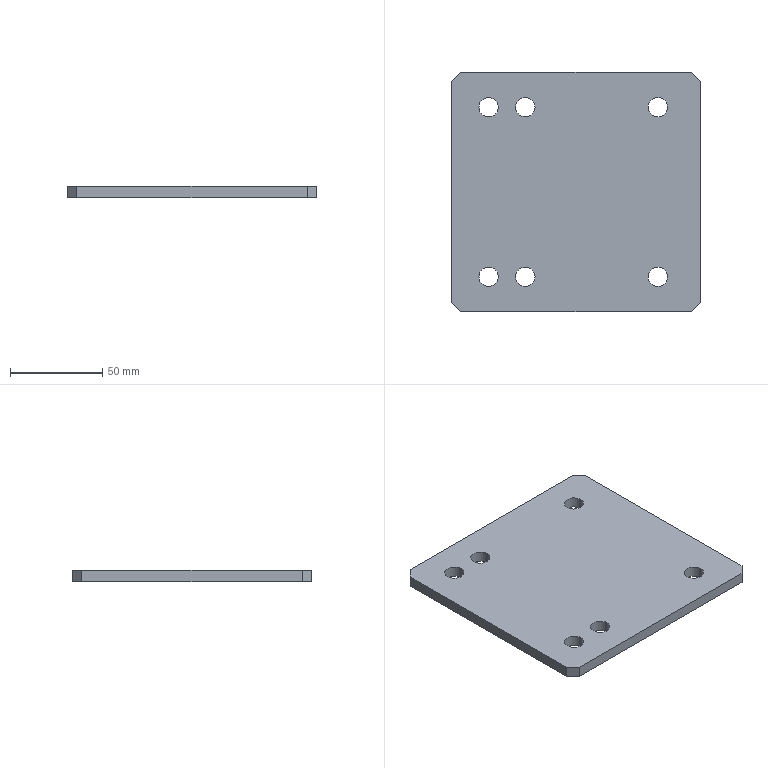Part | SolidWorks | features Extrusion 1 | 1 solid | 22 faces | box 135 x 130 x 6 mm | volume 101883 mm3 | cylinder 12 | plane 10 | commonest cylinder face diameters 10.5 x12
STEP:
#1=CARTESIAN_POINT('',(-52.75,-46.,3.));
#2=VERTEX_POINT('',#1);
#3=CARTESIAN_POINT('',(-42.25,-46.,3.));
#4=VERTEX_POINT('',#3);
#5=CARTESIAN_POINT('',(-47.5,-46.,3.));
#6=DIRECTION('',(0.,0.,1.));
#7=DIRECTION('',(-1.,0.,0.));
#8=AXIS2_PLACEMENT_3D('',#5,#6,#7);
#9=CIRCLE('',#8,5.25);
#10=EDGE_CURVE('',#2,#4,#9,.T.);
#11=ORIENTED_EDGE('',*,*,#10,.T.);
#12=CARTESIAN_POINT('',(-42.25,-46.,-3.));
#13=VERTEX_POINT('',#12);
#14=CARTESIAN_POINT('',(-42.25,-46.,3.));
#15=DIRECTION('',(0.,0.,-1.));
#16=VECTOR('',#15,1000.);
#17=LINE('',#14,#16);
#18=EDGE_CURVE('',#4,#13,#17,.T.);
#19=ORIENTED_EDGE('',*,*,#18,.T.);
#20=CARTESIAN_POINT('',(-52.75,-46.,-3.));
#21=VERTEX_POINT('',#20);
#22=CARTESIAN_POINT('',(-47.5,-46.,-3.));
#23=DIRECTION('',(0.,0.,1.));
#24=DIRECTION('',(-1.,0.,0.));
#25=AXIS2_PLACEMENT_3D('',#22,#23,#24);
#26=CIRCLE('',#25,5.25);
#27=EDGE_CURVE('',#21,#13,#26,.T.);
#28=ORIENTED_EDGE('',*,*,#27,.F.);
#29=CARTESIAN_POINT('',(-52.75,-46.,3.));
#30=DIRECTION('',(0.,0.,-1.));
#31=VECTOR('',#30,1000.);
#32=LINE('',#29,#31);
#33=EDGE_CURVE('',#2,#21,#32,.T.);
#34=ORIENTED_EDGE('',*,*,#33,.F.);
#35=EDGE_LOOP('',(#11,#19,#28,#34));
#36=FACE_OUTER_BOUND('',#35,.T.);
#37=CARTESIAN_POINT('',(-47.5,-46.,3.));
#38=DIRECTION('',(0.,0.,-1.));
#39=DIRECTION('',(-1.,0.,0.));
#40=AXIS2_PLACEMENT_3D('',#37,#38,#39);
#41=CYLINDRICAL_SURFACE('',#40,5.25);
#42=ADVANCED_FACE('',(#36),#41,.F.);
#43=CARTESIAN_POINT('',(-32.75,-46.,3.));
#44=VERTEX_POINT('',#43);
#45=CARTESIAN_POINT('',(-22.25,-46.,3.));
#46=VERTEX_POINT('',#45);
#47=CARTESIAN_POINT('',(-27.5,-46.,3.));
#48=DIRECTION('',(0.,0.,1.));
#49=DIRECTION('',(-1.,0.,0.));
#50=AXIS2_PLACEMENT_3D('',#47,#48,#49);
#51=CIRCLE('',#50,5.25);
#52=EDGE_CURVE('',#44,#46,#51,.T.);
#53=ORIENTED_EDGE('',*,*,#52,.T.);
#54=CARTESIAN_POINT('',(-22.25,-46.,-3.));
#55=VERTEX_POINT('',#54);
#56=CARTESIAN_POINT('',(-22.25,-46.,3.));
#57=DIRECTION('',(0.,0.,-1.));
#58=VECTOR('',#57,1000.);
#59=LINE('',#56,#58);
#60=EDGE_CURVE('',#46,#55,#59,.T.);
#61=ORIENTED_EDGE('',*,*,#60,.T.);
#62=CARTESIAN_POINT('',(-32.75,-46.,-3.));
#63=VERTEX_POINT('',#62);
#64=CARTESIAN_POINT('',(-27.5,-46.,-3.));
#65=DIRECTION('',(0.,0.,1.));
#66=DIRECTION('',(-1.,0.,0.));
#67=AXIS2_PLACEMENT_3D('',#64,#65,#66);
#68=CIRCLE('',#67,5.25);
#69=EDGE_CURVE('',#63,#55,#68,.T.);
#70=ORIENTED_EDGE('',*,*,#69,.F.);
#71=CARTESIAN_POINT('',(-32.75,-46.,3.));
#72=DIRECTION('',(0.,0.,-1.));
#73=VECTOR('',#72,1000.);
#74=LINE('',#71,#73);
#75=EDGE_CURVE('',#44,#63,#74,.T.);
#76=ORIENTED_EDGE('',*,*,#75,.F.);
#77=EDGE_LOOP('',(#53,#61,#70,#76));
#78=FACE_OUTER_BOUND('',#77,.T.);
#79=CARTESIAN_POINT('',(-27.5,-46.,3.));
#80=DIRECTION('',(0.,0.,-1.));
#81=DIRECTION('',(-1.,0.,0.));
#82=AXIS2_PLACEMENT_3D('',#79,#80,#81);
#83=CYLINDRICAL_SURFACE('',#82,5.25);
#84=ADVANCED_FACE('',(#78),#83,.F.);
#85=CARTESIAN_POINT('',(39.25,-46.,3.));
#86=VERTEX_POINT('',#85);
#87=CARTESIAN_POINT('',(49.75,-46.,3.));
#88=VERTEX_POINT('',#87);
#89=CARTESIAN_POINT('',(44.5,-46.,3.));
#90=DIRECTION('',(0.,0.,1.));
#91=DIRECTION('',(-1.,0.,0.));
#92=AXIS2_PLACEMENT_3D('',#89,#90,#91);
#93=CIRCLE('',#92,5.25);
#94=EDGE_CURVE('',#86,#88,#93,.T.);
#95=ORIENTED_EDGE('',*,*,#94,.T.);
#96=CARTESIAN_POINT('',(49.75,-46.,-3.));
#97=VERTEX_POINT('',#96);
#98=CARTESIAN_POINT('',(49.75,-46.,3.));
#99=DIRECTION('',(0.,0.,-1.));
#100=VECTOR('',#99,1000.);
#101=LINE('',#98,#100);
#102=EDGE_CURVE('',#88,#97,#101,.T.);
#103=ORIENTED_EDGE('',*,*,#102,.T.);
#104=CARTESIAN_POINT('',(39.25,-46.,-3.));
#105=VERTEX_POINT('',#104);
#106=CARTESIAN_POINT('',(44.5,-46.,-3.));
#107=DIRECTION('',(0.,0.,1.));
#108=DIRECTION('',(-1.,0.,0.));
#109=AXIS2_PLACEMENT_3D('',#106,#107,#108);
#110=CIRCLE('',#109,5.25);
#111=EDGE_CURVE('',#105,#97,#110,.T.);
#112=ORIENTED_EDGE('',*,*,#111,.F.);
#113=CARTESIAN_POINT('',(39.25,-46.,3.));
#114=DIRECTION('',(0.,0.,-1.));
#115=VECTOR('',#114,1000.);
#116=LINE('',#113,#115);
#117=EDGE_CURVE('',#86,#105,#116,.T.);
#118=ORIENTED_EDGE('',*,*,#117,.F.);
#119=EDGE_LOOP('',(#95,#103,#112,#118));
#120=FACE_OUTER_BOUND('',#119,.T.);
#121=CARTESIAN_POINT('',(44.5,-46.,3.));
#122=DIRECTION('',(0.,0.,-1.));
#123=DIRECTION('',(-1.,0.,0.));
#124=AXIS2_PLACEMENT_3D('',#121,#122,#123);
#125=CYLINDRICAL_SURFACE('',#124,5.25);
#126=ADVANCED_FACE('',(#120),#125,.F.);
#127=CARTESIAN_POINT('',(39.25,46.,3.));
#128=VERTEX_POINT('',#127);
#129=CARTESIAN_POINT('',(49.75,46.,3.));
#130=VERTEX_POINT('',#129);
#131=CARTESIAN_POINT('',(44.5,46.,3.));
#132=DIRECTION('',(0.,0.,1.));
#133=DIRECTION('',(1.,0.,0.));
#134=AXIS2_PLACEMENT_3D('',#131,#132,#133);
#135=CIRCLE('',#134,5.25);
#136=EDGE_CURVE('',#128,#130,#135,.T.);
#137=ORIENTED_EDGE('',*,*,#136,.T.);
#138=CARTESIAN_POINT('',(49.75,46.,-3.));
#139=VERTEX_POINT('',#138);
#140=CARTESIAN_POINT('',(49.75,46.,3.));
#141=DIRECTION('',(0.,0.,-1.));
#142=VECTOR('',#141,1000.);
#143=LINE('',#140,#142);
#144=EDGE_CURVE('',#130,#139,#143,.T.);
#145=ORIENTED_EDGE('',*,*,#144,.T.);
#146=CARTESIAN_POINT('',(39.25,46.,-3.));
#147=VERTEX_POINT('',#146);
#148=CARTESIAN_POINT('',(44.5,46.,-3.));
#149=DIRECTION('',(0.,0.,1.));
#150=DIRECTION('',(1.,0.,0.));
#151=AXIS2_PLACEMENT_3D('',#148,#149,#150);
#152=CIRCLE('',#151,5.25);
#153=EDGE_CURVE('',#147,#139,#152,.T.);
#154=ORIENTED_EDGE('',*,*,#153,.F.);
#155=CARTESIAN_POINT('',(39.25,46.,3.));
#156=DIRECTION('',(0.,0.,-1.));
#157=VECTOR('',#156,1000.);
#158=LINE('',#155,#157);
#159=EDGE_CURVE('',#128,#147,#158,.T.);
#160=ORIENTED_EDGE('',*,*,#159,.F.);
#161=EDGE_LOOP('',(#137,#145,#154,#160));
#162=FACE_OUTER_BOUND('',#161,.T.);
#163=CARTESIAN_POINT('',(44.5,46.,3.));
#164=DIRECTION('',(0.,0.,-1.));
#165=DIRECTION('',(-1.,0.,0.));
#166=AXIS2_PLACEMENT_3D('',#163,#164,#165);
#167=CYLINDRICAL_SURFACE('',#166,5.25);
#168=ADVANCED_FACE('',(#162),#167,.F.);
#169=CARTESIAN_POINT('',(-32.75,46.,3.));
#170=VERTEX_POINT('',#169);
#171=CARTESIAN_POINT('',(-22.25,46.,3.));
#172=VERTEX_POINT('',#171);
#173=CARTESIAN_POINT('',(-27.5,46.,3.));
#174=DIRECTION('',(0.,0.,1.));
#175=DIRECTION('',(1.,0.,0.));
#176=AXIS2_PLACEMENT_3D('',#173,#174,#175);
#177=CIRCLE('',#176,5.25);
#178=EDGE_CURVE('',#170,#172,#177,.T.);
#179=ORIENTED_EDGE('',*,*,#178,.T.);
#180=CARTESIAN_POINT('',(-22.25,46.,-3.));
#181=VERTEX_POINT('',#180);
#182=CARTESIAN_POINT('',(-22.25,46.,3.));
#183=DIRECTION('',(0.,0.,-1.));
#184=VECTOR('',#183,1000.);
#185=LINE('',#182,#184);
#186=EDGE_CURVE('',#172,#181,#185,.T.);
#187=ORIENTED_EDGE('',*,*,#186,.T.);
#188=CARTESIAN_POINT('',(-32.75,46.,-3.));
#189=VERTEX_POINT('',#188);
#190=CARTESIAN_POINT('',(-27.5,46.,-3.));
#191=DIRECTION('',(0.,0.,1.));
#192=DIRECTION('',(1.,0.,0.));
#193=AXIS2_PLACEMENT_3D('',#190,#191,#192);
#194=CIRCLE('',#193,5.25);
#195=EDGE_CURVE('',#189,#181,#194,.T.);
#196=ORIENTED_EDGE('',*,*,#195,.F.);
#197=CARTESIAN_POINT('',(-32.75,46.,3.));
#198=DIRECTION('',(0.,0.,-1.));
#199=VECTOR('',#198,1000.);
#200=LINE('',#197,#199);
#201=EDGE_CURVE('',#170,#189,#200,.T.);
#202=ORIENTED_EDGE('',*,*,#201,.F.);
#203=EDGE_LOOP('',(#179,#187,#196,#202));
#204=FACE_OUTER_BOUND('',#203,.T.);
#205=CARTESIAN_POINT('',(-27.5,46.,3.));
#206=DIRECTION('',(0.,0.,-1.));
#207=DIRECTION('',(-1.,0.,0.));
#208=AXIS2_PLACEMENT_3D('',#205,#206,#207);
#209=CYLINDRICAL_SURFACE('',#208,5.25);
#210=ADVANCED_FACE('',(#204),#209,.F.);
#211=CARTESIAN_POINT('',(-52.75,46.,3.));
#212=VERTEX_POINT('',#211);
#213=CARTESIAN_POINT('',(-42.25,46.,3.));
#214=VERTEX_POINT('',#213);
#215=CARTESIAN_POINT('',(-47.5,46.,3.));
#216=DIRECTION('',(0.,0.,1.));
#217=DIRECTION('',(1.,0.,0.));
#218=AXIS2_PLACEMENT_3D('',#215,#216,#217);
#219=CIRCLE('',#218,5.25);
#220=EDGE_CURVE('',#212,#214,#219,.T.);
#221=ORIENTED_EDGE('',*,*,#220,.T.);
#222=CARTESIAN_POINT('',(-42.25,46.,-3.));
#223=VERTEX_POINT('',#222);
#224=CARTESIAN_POINT('',(-42.25,46.,3.));
#225=DIRECTION('',(0.,0.,-1.));
#226=VECTOR('',#225,1000.);
#227=LINE('',#224,#226);
#228=EDGE_CURVE('',#214,#223,#227,.T.);
#229=ORIENTED_EDGE('',*,*,#228,.T.);
#230=CARTESIAN_POINT('',(-52.75,46.,-3.));
#231=VERTEX_POINT('',#230);
#232=CARTESIAN_POINT('',(-47.5,46.,-3.));
#233=DIRECTION('',(0.,0.,1.));
#234=DIRECTION('',(1.,0.,0.));
#235=AXIS2_PLACEMENT_3D('',#232,#233,#234);
#236=CIRCLE('',#235,5.25);
#237=EDGE_CURVE('',#231,#223,#236,.T.);
#238=ORIENTED_EDGE('',*,*,#237,.F.);
#239=CARTESIAN_POINT('',(-52.75,46.,3.));
#240=DIRECTION('',(0.,0.,-1.));
#241=VECTOR('',#240,1000.);
#242=LINE('',#239,#241);
#243=EDGE_CURVE('',#212,#231,#242,.T.);
#244=ORIENTED_EDGE('',*,*,#243,.F.);
#245=EDGE_LOOP('',(#221,#229,#238,#244));
#246=FACE_OUTER_BOUND('',#245,.T.);
#247=CARTESIAN_POINT('',(-47.5,46.,3.));
#248=DIRECTION('',(0.,0.,-1.));
#249=DIRECTION('',(-1.,0.,0.));
#250=AXIS2_PLACEMENT_3D('',#247,#248,#249);
#251=CYLINDRICAL_SURFACE('',#250,5.25);
#252=ADVANCED_FACE('',(#246),#251,.F.);
#253=ORIENTED_EDGE('',*,*,#52,.F.);
#254=CARTESIAN_POINT('',(-27.5,-46.,3.));
#255=DIRECTION('',(0.,0.,1.));
#256=DIRECTION('',(-1.,0.,0.));
#257=AXIS2_PLACEMENT_3D('',#254,#255,#256);
#258=CIRCLE('',#257,5.25);
#259=EDGE_CURVE('',#46,#44,#258,.T.);
#260=ORIENTED_EDGE('',*,*,#259,.F.);
#261=EDGE_LOOP('',(#253,#260));
#262=FACE_BOUND('',#261,.T.);
#263=ORIENTED_EDGE('',*,*,#136,.F.);
#264=CARTESIAN_POINT('',(44.5,46.,3.));
#265=DIRECTION('',(0.,0.,1.));
#266=DIRECTION('',(1.,0.,0.));
#267=AXIS2_PLACEMENT_3D('',#264,#265,#266);
#268=CIRCLE('',#267,5.25);
#269=EDGE_CURVE('',#130,#128,#268,.T.);
#270=ORIENTED_EDGE('',*,*,#269,.F.);
#271=EDGE_LOOP('',(#263,#270));
#272=FACE_BOUND('',#271,.T.);
#273=ORIENTED_EDGE('',*,*,#220,.F.);
#274=CARTESIAN_POINT('',(-47.5,46.,3.));
#275=DIRECTION('',(0.,0.,1.));
#276=DIRECTION('',(1.,0.,0.));
#277=AXIS2_PLACEMENT_3D('',#274,#275,#276);
#278=CIRCLE('',#277,5.25);
#279=EDGE_CURVE('',#214,#212,#278,.T.);
#280=ORIENTED_EDGE('',*,*,#279,.F.);
#281=EDGE_LOOP('',(#273,#280));
#282=FACE_BOUND('',#281,.T.);
#283=CARTESIAN_POINT('',(-67.5,60.,3.));
#284=VERTEX_POINT('',#283);
#285=CARTESIAN_POINT('',(-67.5,-60.,3.));
#286=VERTEX_POINT('',#285);
#287=CARTESIAN_POINT('',(-67.5,-60.,3.));
#288=DIRECTION('',(0.,-1.,0.));
#289=VECTOR('',#288,1000.);
#290=LINE('',#287,#289);
#291=EDGE_CURVE('',#284,#286,#290,.T.);
#292=ORIENTED_EDGE('',*,*,#291,.T.);
#293=CARTESIAN_POINT('',(-62.5,-65.,3.));
#294=VERTEX_POINT('',#293);
#295=CARTESIAN_POINT('',(-62.5,-65.,3.));
#296=DIRECTION('',(0.7071,-0.7071,0.));
#297=VECTOR('',#296,1000.);
#298=LINE('',#295,#297);
#299=EDGE_CURVE('',#286,#294,#298,.T.);
#300=ORIENTED_EDGE('',*,*,#299,.T.);
#301=CARTESIAN_POINT('',(62.5,-65.,3.));
#302=VERTEX_POINT('',#301);
#303=CARTESIAN_POINT('',(62.5,-65.,3.));
#304=DIRECTION('',(1.,0.,0.));
#305=VECTOR('',#304,1000.);
#306=LINE('',#303,#305);
#307=EDGE_CURVE('',#294,#302,#306,.T.);
#308=ORIENTED_EDGE('',*,*,#307,.T.);
#309=CARTESIAN_POINT('',(67.5,-60.,3.));
#310=VERTEX_POINT('',#309);
#311=CARTESIAN_POINT('',(62.5,-65.,3.));
#312=DIRECTION('',(0.7071,0.7071,0.));
#313=VECTOR('',#312,1000.);
#314=LINE('',#311,#313);
#315=EDGE_CURVE('',#302,#310,#314,.T.);
#316=ORIENTED_EDGE('',*,*,#315,.T.);
#317=CARTESIAN_POINT('',(67.5,60.,3.));
#318=VERTEX_POINT('',#317);
#319=CARTESIAN_POINT('',(67.5,-60.,3.));
#320=DIRECTION('',(0.,1.,0.));
#321=VECTOR('',#320,1000.);
#322=LINE('',#319,#321);
#323=EDGE_CURVE('',#310,#318,#322,.T.);
#324=ORIENTED_EDGE('',*,*,#323,.T.);
#325=CARTESIAN_POINT('',(62.5,65.,3.));
#326=VERTEX_POINT('',#325);
#327=CARTESIAN_POINT('',(67.5,60.,3.));
#328=DIRECTION('',(-0.7071,0.7071,0.));
#329=VECTOR('',#328,1000.);
#330=LINE('',#327,#329);
#331=EDGE_CURVE('',#318,#326,#330,.T.);
#332=ORIENTED_EDGE('',*,*,#331,.T.);
#333=CARTESIAN_POINT('',(-62.5,65.,3.));
#334=VERTEX_POINT('',#333);
#335=CARTESIAN_POINT('',(62.5,65.,3.));
#336=DIRECTION('',(-1.,0.,0.));
#337=VECTOR('',#336,1000.);
#338=LINE('',#335,#337);
#339=EDGE_CURVE('',#326,#334,#338,.T.);
#340=ORIENTED_EDGE('',*,*,#339,.T.);
#341=CARTESIAN_POINT('',(-67.5,60.,3.));
#342=DIRECTION('',(-0.7071,-0.7071,0.));
#343=VECTOR('',#342,1000.);
#344=LINE('',#341,#343);
#345=EDGE_CURVE('',#334,#284,#344,.T.);
#346=ORIENTED_EDGE('',*,*,#345,.T.);
#347=EDGE_LOOP('',(#292,#300,#308,#316,#324,#332,#340,#346));
#348=FACE_OUTER_BOUND('',#347,.T.);
#349=ORIENTED_EDGE('',*,*,#178,.F.);
#350=CARTESIAN_POINT('',(-27.5,46.,3.));
#351=DIRECTION('',(0.,0.,1.));
#352=DIRECTION('',(1.,0.,0.));
#353=AXIS2_PLACEMENT_3D('',#350,#351,#352);
#354=CIRCLE('',#353,5.25);
#355=EDGE_CURVE('',#172,#170,#354,.T.);
#356=ORIENTED_EDGE('',*,*,#355,.F.);
#357=EDGE_LOOP('',(#349,#356));
#358=FACE_BOUND('',#357,.T.);
#359=ORIENTED_EDGE('',*,*,#94,.F.);
#360=CARTESIAN_POINT('',(44.5,-46.,3.));
#361=DIRECTION('',(0.,0.,1.));
#362=DIRECTION('',(-1.,0.,0.));
#363=AXIS2_PLACEMENT_3D('',#360,#361,#362);
#364=CIRCLE('',#363,5.25);
#365=EDGE_CURVE('',#88,#86,#364,.T.);
#366=ORIENTED_EDGE('',*,*,#365,.F.);
#367=EDGE_LOOP('',(#359,#366));
#368=FACE_BOUND('',#367,.T.);
#369=ORIENTED_EDGE('',*,*,#10,.F.);
#370=CARTESIAN_POINT('',(-47.5,-46.,3.));
#371=DIRECTION('',(0.,0.,1.));
#372=DIRECTION('',(-1.,0.,0.));
#373=AXIS2_PLACEMENT_3D('',#370,#371,#372);
#374=CIRCLE('',#373,5.25);
#375=EDGE_CURVE('',#4,#2,#374,.T.);
#376=ORIENTED_EDGE('',*,*,#375,.F.);
#377=EDGE_LOOP('',(#369,#376));
#378=FACE_BOUND('',#377,.T.);
#379=CARTESIAN_POINT('',(0.,0.,3.));
#380=DIRECTION('',(0.,0.,1.));
#381=DIRECTION('',(1.,0.,0.));
#382=AXIS2_PLACEMENT_3D('',#379,#380,#381);
#383=PLANE('',#382);
#384=ADVANCED_FACE('',(#262,#272,#282,#348,#358,#368,#378),#383,.T.);
#385=CARTESIAN_POINT('',(-67.5,60.,-3.));
#386=VERTEX_POINT('',#385);
#387=CARTESIAN_POINT('',(-67.5,-60.,-3.));
#388=VERTEX_POINT('',#387);
#389=CARTESIAN_POINT('',(-67.5,-60.,-3.));
#390=DIRECTION('',(0.,-1.,0.));
#391=VECTOR('',#390,1000.);
#392=LINE('',#389,#391);
#393=EDGE_CURVE('',#386,#388,#392,.T.);
#394=ORIENTED_EDGE('',*,*,#393,.F.);
#395=CARTESIAN_POINT('',(-62.5,65.,-3.));
#396=VERTEX_POINT('',#395);
#397=CARTESIAN_POINT('',(-67.5,60.,-3.));
#398=DIRECTION('',(-0.7071,-0.7071,0.));
#399=VECTOR('',#398,1000.);
#400=LINE('',#397,#399);
#401=EDGE_CURVE('',#396,#386,#400,.T.);
#402=ORIENTED_EDGE('',*,*,#401,.F.);
#403=CARTESIAN_POINT('',(62.5,65.,-3.));
#404=VERTEX_POINT('',#403);
#405=CARTESIAN_POINT('',(62.5,65.,-3.));
#406=DIRECTION('',(-1.,0.,0.));
#407=VECTOR('',#406,1000.);
#408=LINE('',#405,#407);
#409=EDGE_CURVE('',#404,#396,#408,.T.);
#410=ORIENTED_EDGE('',*,*,#409,.F.);
#411=CARTESIAN_POINT('',(67.5,60.,-3.));
#412=VERTEX_POINT('',#411);
#413=CARTESIAN_POINT('',(67.5,60.,-3.));
#414=DIRECTION('',(-0.7071,0.7071,0.));
#415=VECTOR('',#414,1000.);
#416=LINE('',#413,#415);
#417=EDGE_CURVE('',#412,#404,#416,.T.);
#418=ORIENTED_EDGE('',*,*,#417,.F.);
#419=CARTESIAN_POINT('',(67.5,-60.,-3.));
#420=VERTEX_POINT('',#419);
#421=CARTESIAN_POINT('',(67.5,-60.,-3.));
#422=DIRECTION('',(0.,1.,0.));
#423=VECTOR('',#422,1000.);
#424=LINE('',#421,#423);
#425=EDGE_CURVE('',#420,#412,#424,.T.);
#426=ORIENTED_EDGE('',*,*,#425,.F.);
#427=CARTESIAN_POINT('',(62.5,-65.,-3.));
#428=VERTEX_POINT('',#427);
#429=CARTESIAN_POINT('',(62.5,-65.,-3.));
#430=DIRECTION('',(0.7071,0.7071,0.));
#431=VECTOR('',#430,1000.);
#432=LINE('',#429,#431);
#433=EDGE_CURVE('',#428,#420,#432,.T.);
#434=ORIENTED_EDGE('',*,*,#433,.F.);
#435=CARTESIAN_POINT('',(-62.5,-65.,-3.));
#436=VERTEX_POINT('',#435);
#437=CARTESIAN_POINT('',(62.5,-65.,-3.));
#438=DIRECTION('',(1.,0.,0.));
#439=VECTOR('',#438,1000.);
#440=LINE('',#437,#439);
#441=EDGE_CURVE('',#436,#428,#440,.T.);
#442=ORIENTED_EDGE('',*,*,#441,.F.);
#443=CARTESIAN_POINT('',(-62.5,-65.,-3.));
#444=DIRECTION('',(0.7071,-0.7071,0.));
#445=VECTOR('',#444,1000.);
#446=LINE('',#443,#445);
#447=EDGE_CURVE('',#388,#436,#446,.T.);
#448=ORIENTED_EDGE('',*,*,#447,.F.);
#449=EDGE_LOOP('',(#394,#402,#410,#418,#426,#434,#442,#448));
#450=FACE_OUTER_BOUND('',#449,.T.);
#451=ORIENTED_EDGE('',*,*,#237,.T.);
#452=CARTESIAN_POINT('',(-47.5,46.,-3.));
#453=DIRECTION('',(0.,0.,1.));
#454=DIRECTION('',(1.,0.,0.));
#455=AXIS2_PLACEMENT_3D('',#452,#453,#454);
#456=CIRCLE('',#455,5.25);
#457=EDGE_CURVE('',#223,#231,#456,.T.);
#458=ORIENTED_EDGE('',*,*,#457,.T.);
#459=EDGE_LOOP('',(#451,#458));
#460=FACE_BOUND('',#459,.T.);
#461=ORIENTED_EDGE('',*,*,#195,.T.);
#462=CARTESIAN_POINT('',(-27.5,46.,-3.));
#463=DIRECTION('',(0.,0.,1.));
#464=DIRECTION('',(1.,0.,0.));
#465=AXIS2_PLACEMENT_3D('',#462,#463,#464);
#466=CIRCLE('',#465,5.25);
#467=EDGE_CURVE('',#181,#189,#466,.T.);
#468=ORIENTED_EDGE('',*,*,#467,.T.);
#469=EDGE_LOOP('',(#461,#468));
#470=FACE_BOUND('',#469,.T.);
#471=ORIENTED_EDGE('',*,*,#153,.T.);
#472=CARTESIAN_POINT('',(44.5,46.,-3.));
#473=DIRECTION('',(0.,0.,1.));
#474=DIRECTION('',(1.,0.,0.));
#475=AXIS2_PLACEMENT_3D('',#472,#473,#474);
#476=CIRCLE('',#475,5.25);
#477=EDGE_CURVE('',#139,#147,#476,.T.);
#478=ORIENTED_EDGE('',*,*,#477,.T.);
#479=EDGE_LOOP('',(#471,#478));
#480=FACE_BOUND('',#479,.T.);
#481=ORIENTED_EDGE('',*,*,#111,.T.);
#482=CARTESIAN_POINT('',(44.5,-46.,-3.));
#483=DIRECTION('',(0.,0.,1.));
#484=DIRECTION('',(-1.,0.,0.));
#485=AXIS2_PLACEMENT_3D('',#482,#483,#484);
#486=CIRCLE('',#485,5.25);
#487=EDGE_CURVE('',#97,#105,#486,.T.);
#488=ORIENTED_EDGE('',*,*,#487,.T.);
#489=EDGE_LOOP('',(#481,#488));
#490=FACE_BOUND('',#489,.T.);
#491=ORIENTED_EDGE('',*,*,#69,.T.);
#492=CARTESIAN_POINT('',(-27.5,-46.,-3.));
#493=DIRECTION('',(0.,0.,1.));
#494=DIRECTION('',(-1.,0.,0.));
#495=AXIS2_PLACEMENT_3D('',#492,#493,#494);
#496=CIRCLE('',#495,5.25);
#497=EDGE_CURVE('',#55,#63,#496,.T.);
#498=ORIENTED_EDGE('',*,*,#497,.T.);
#499=EDGE_LOOP('',(#491,#498));
#500=FACE_BOUND('',#499,.T.);
#501=ORIENTED_EDGE('',*,*,#27,.T.);
#502=CARTESIAN_POINT('',(-47.5,-46.,-3.));
#503=DIRECTION('',(0.,0.,1.));
#504=DIRECTION('',(-1.,0.,0.));
#505=AXIS2_PLACEMENT_3D('',#502,#503,#504);
#506=CIRCLE('',#505,5.25);
#507=EDGE_CURVE('',#13,#21,#506,.T.);
#508=ORIENTED_EDGE('',*,*,#507,.T.);
#509=EDGE_LOOP('',(#501,#508));
#510=FACE_BOUND('',#509,.T.);
#511=CARTESIAN_POINT('',(0.,0.,-3.));
#512=DIRECTION('',(0.,0.,1.));
#513=DIRECTION('',(1.,0.,0.));
#514=AXIS2_PLACEMENT_3D('',#511,#512,#513);
#515=PLANE('',#514);
#516=ADVANCED_FACE('',(#450,#460,#470,#480,#490,#500,#510),#515,.F.);
#517=ORIENTED_EDGE('',*,*,#393,.T.);
#518=CARTESIAN_POINT('',(-67.5,-60.,3.));
#519=DIRECTION('',(0.,0.,-1.));
#520=VECTOR('',#519,1000.);
#521=LINE('',#518,#520);
#522=EDGE_CURVE('',#286,#388,#521,.T.);
#523=ORIENTED_EDGE('',*,*,#522,.F.);
#524=ORIENTED_EDGE('',*,*,#291,.F.);
#525=CARTESIAN_POINT('',(-67.5,60.,3.));
#526=DIRECTION('',(0.,0.,-1.));
#527=VECTOR('',#526,1000.);
#528=LINE('',#525,#527);
#529=EDGE_CURVE('',#284,#386,#528,.T.);
#530=ORIENTED_EDGE('',*,*,#529,.T.);
#531=EDGE_LOOP('',(#517,#523,#524,#530));
#532=FACE_OUTER_BOUND('',#531,.T.);
#533=CARTESIAN_POINT('',(-67.5,-60.,3.));
#534=DIRECTION('',(1.,0.,0.));
#535=DIRECTION('',(0.,1.,0.));
#536=AXIS2_PLACEMENT_3D('',#533,#534,#535);
#537=PLANE('',#536);
#538=ADVANCED_FACE('',(#532),#537,.F.);
#539=ORIENTED_EDGE('',*,*,#447,.T.);
#540=CARTESIAN_POINT('',(-62.5,-65.,3.));
#541=DIRECTION('',(0.,0.,-1.));
#542=VECTOR('',#541,1000.);
#543=LINE('',#540,#542);
#544=EDGE_CURVE('',#294,#436,#543,.T.);
#545=ORIENTED_EDGE('',*,*,#544,.F.);
#546=ORIENTED_EDGE('',*,*,#299,.F.);
#547=ORIENTED_EDGE('',*,*,#522,.T.);
#548=EDGE_LOOP('',(#539,#545,#546,#547));
#549=FACE_OUTER_BOUND('',#548,.T.);
#550=CARTESIAN_POINT('',(-62.5,-65.,3.));
#551=DIRECTION('',(0.7071,0.7071,0.));
#552=DIRECTION('',(-0.7071,0.7071,0.));
#553=AXIS2_PLACEMENT_3D('',#550,#551,#552);
#554=PLANE('',#553);
#555=ADVANCED_FACE('',(#549),#554,.F.);
#556=ORIENTED_EDGE('',*,*,#441,.T.);
#557=CARTESIAN_POINT('',(62.5,-65.,3.));
#558=DIRECTION('',(0.,0.,-1.));
#559=VECTOR('',#558,1000.);
#560=LINE('',#557,#559);
#561=EDGE_CURVE('',#302,#428,#560,.T.);
#562=ORIENTED_EDGE('',*,*,#561,.F.);
#563=ORIENTED_EDGE('',*,*,#307,.F.);
#564=ORIENTED_EDGE('',*,*,#544,.T.);
#565=EDGE_LOOP('',(#556,#562,#563,#564));
#566=FACE_OUTER_BOUND('',#565,.T.);
#567=CARTESIAN_POINT('',(62.5,-65.,3.));
#568=DIRECTION('',(0.,1.,0.));
#569=DIRECTION('',(-1.,0.,0.));
#570=AXIS2_PLACEMENT_3D('',#567,#568,#569);
#571=PLANE('',#570);
#572=ADVANCED_FACE('',(#566),#571,.F.);
#573=ORIENTED_EDGE('',*,*,#433,.T.);
#574=CARTESIAN_POINT('',(67.5,-60.,3.));
#575=DIRECTION('',(0.,0.,-1.));
#576=VECTOR('',#575,1000.);
#577=LINE('',#574,#576);
#578=EDGE_CURVE('',#310,#420,#577,.T.);
#579=ORIENTED_EDGE('',*,*,#578,.F.);
#580=ORIENTED_EDGE('',*,*,#315,.F.);
#581=ORIENTED_EDGE('',*,*,#561,.T.);
#582=EDGE_LOOP('',(#573,#579,#580,#581));
#583=FACE_OUTER_BOUND('',#582,.T.);
#584=CARTESIAN_POINT('',(62.5,-65.,3.));
#585=DIRECTION('',(-0.7071,0.7071,0.));
#586=DIRECTION('',(-0.7071,-0.7071,0.));
#587=AXIS2_PLACEMENT_3D('',#584,#585,#586);
#588=PLANE('',#587);
#589=ADVANCED_FACE('',(#583),#588,.F.);
#590=ORIENTED_EDGE('',*,*,#425,.T.);
#591=CARTESIAN_POINT('',(67.5,60.,3.));
#592=DIRECTION('',(0.,0.,-1.));
#593=VECTOR('',#592,1000.);
#594=LINE('',#591,#593);
#595=EDGE_CURVE('',#318,#412,#594,.T.);
#596=ORIENTED_EDGE('',*,*,#595,.F.);
#597=ORIENTED_EDGE('',*,*,#323,.F.);
#598=ORIENTED_EDGE('',*,*,#578,.T.);
#599=EDGE_LOOP('',(#590,#596,#597,#598));
#600=FACE_OUTER_BOUND('',#599,.T.);
#601=CARTESIAN_POINT('',(67.5,-60.,3.));
#602=DIRECTION('',(-1.,0.,0.));
#603=DIRECTION('',(0.,0.,1.));
#604=AXIS2_PLACEMENT_3D('',#601,#602,#603);
#605=PLANE('',#604);
#606=ADVANCED_FACE('',(#600),#605,.F.);
#607=ORIENTED_EDGE('',*,*,#417,.T.);
#608=CARTESIAN_POINT('',(62.5,65.,3.));
#609=DIRECTION('',(0.,0.,-1.));
#610=VECTOR('',#609,1000.);
#611=LINE('',#608,#610);
#612=EDGE_CURVE('',#326,#404,#611,.T.);
#613=ORIENTED_EDGE('',*,*,#612,.F.);
#614=ORIENTED_EDGE('',*,*,#331,.F.);
#615=ORIENTED_EDGE('',*,*,#595,.T.);
#616=EDGE_LOOP('',(#607,#613,#614,#615));
#617=FACE_OUTER_BOUND('',#616,.T.);
#618=CARTESIAN_POINT('',(67.5,60.,3.));
#619=DIRECTION('',(-0.7071,-0.7071,0.));
#620=DIRECTION('',(0.7071,-0.7071,0.));
#621=AXIS2_PLACEMENT_3D('',#618,#619,#620);
#622=PLANE('',#621);
#623=ADVANCED_FACE('',(#617),#622,.F.);
#624=ORIENTED_EDGE('',*,*,#409,.T.);
#625=CARTESIAN_POINT('',(-62.5,65.,3.));
#626=DIRECTION('',(0.,0.,-1.));
#627=VECTOR('',#626,1000.);
#628=LINE('',#625,#627);
#629=EDGE_CURVE('',#334,#396,#628,.T.);
#630=ORIENTED_EDGE('',*,*,#629,.F.);
#631=ORIENTED_EDGE('',*,*,#339,.F.);
#632=ORIENTED_EDGE('',*,*,#612,.T.);
#633=EDGE_LOOP('',(#624,#630,#631,#632));
#634=FACE_OUTER_BOUND('',#633,.T.);
#635=CARTESIAN_POINT('',(62.5,65.,3.));
#636=DIRECTION('',(0.,-1.,0.));
#637=DIRECTION('',(1.,0.,0.));
#638=AXIS2_PLACEMENT_3D('',#635,#636,#637);
#639=PLANE('',#638);
#640=ADVANCED_FACE('',(#634),#639,.F.);
#641=ORIENTED_EDGE('',*,*,#401,.T.);
#642=ORIENTED_EDGE('',*,*,#529,.F.);
#643=ORIENTED_EDGE('',*,*,#345,.F.);
#644=ORIENTED_EDGE('',*,*,#629,.T.);
#645=EDGE_LOOP('',(#641,#642,#643,#644));
#646=FACE_OUTER_BOUND('',#645,.T.);
#647=CARTESIAN_POINT('',(-67.5,60.,3.));
#648=DIRECTION('',(0.7071,-0.7071,0.));
#649=DIRECTION('',(0.7071,0.7071,0.));
#650=AXIS2_PLACEMENT_3D('',#647,#648,#649);
#651=PLANE('',#650);
#652=ADVANCED_FACE('',(#646),#651,.F.);
#653=ORIENTED_EDGE('',*,*,#228,.F.);
#654=ORIENTED_EDGE('',*,*,#279,.T.);
#655=ORIENTED_EDGE('',*,*,#243,.T.);
#656=ORIENTED_EDGE('',*,*,#457,.F.);
#657=EDGE_LOOP('',(#653,#654,#655,#656));
#658=FACE_OUTER_BOUND('',#657,.T.);
#659=CARTESIAN_POINT('',(-47.5,46.,3.));
#660=DIRECTION('',(0.,0.,-1.));
#661=DIRECTION('',(-1.,0.,0.));
#662=AXIS2_PLACEMENT_3D('',#659,#660,#661);
#663=CYLINDRICAL_SURFACE('',#662,5.25);
#664=ADVANCED_FACE('',(#658),#663,.F.);
#665=ORIENTED_EDGE('',*,*,#186,.F.);
#666=ORIENTED_EDGE('',*,*,#355,.T.);
#667=ORIENTED_EDGE('',*,*,#201,.T.);
#668=ORIENTED_EDGE('',*,*,#467,.F.);
#669=EDGE_LOOP('',(#665,#666,#667,#668));
#670=FACE_OUTER_BOUND('',#669,.T.);
#671=CARTESIAN_POINT('',(-27.5,46.,3.));
#672=DIRECTION('',(0.,0.,-1.));
#673=DIRECTION('',(-1.,0.,0.));
#674=AXIS2_PLACEMENT_3D('',#671,#672,#673);
#675=CYLINDRICAL_SURFACE('',#674,5.25);
#676=ADVANCED_FACE('',(#670),#675,.F.);
#677=ORIENTED_EDGE('',*,*,#144,.F.);
#678=ORIENTED_EDGE('',*,*,#269,.T.);
#679=ORIENTED_EDGE('',*,*,#159,.T.);
#680=ORIENTED_EDGE('',*,*,#477,.F.);
#681=EDGE_LOOP('',(#677,#678,#679,#680));
#682=FACE_OUTER_BOUND('',#681,.T.);
#683=CARTESIAN_POINT('',(44.5,46.,3.));
#684=DIRECTION('',(0.,0.,-1.));
#685=DIRECTION('',(-1.,0.,0.));
#686=AXIS2_PLACEMENT_3D('',#683,#684,#685);
#687=CYLINDRICAL_SURFACE('',#686,5.25);
#688=ADVANCED_FACE('',(#682),#687,.F.);
#689=ORIENTED_EDGE('',*,*,#102,.F.);
#690=ORIENTED_EDGE('',*,*,#365,.T.);
#691=ORIENTED_EDGE('',*,*,#117,.T.);
#692=ORIENTED_EDGE('',*,*,#487,.F.);
#693=EDGE_LOOP('',(#689,#690,#691,#692));
#694=FACE_OUTER_BOUND('',#693,.T.);
#695=CARTESIAN_POINT('',(44.5,-46.,3.));
#696=DIRECTION('',(0.,0.,-1.));
#697=DIRECTION('',(-1.,0.,0.));
#698=AXIS2_PLACEMENT_3D('',#695,#696,#697);
#699=CYLINDRICAL_SURFACE('',#698,5.25);
#700=ADVANCED_FACE('',(#694),#699,.F.);
#701=ORIENTED_EDGE('',*,*,#60,.F.);
#702=ORIENTED_EDGE('',*,*,#259,.T.);
#703=ORIENTED_EDGE('',*,*,#75,.T.);
#704=ORIENTED_EDGE('',*,*,#497,.F.);
#705=EDGE_LOOP('',(#701,#702,#703,#704));
#706=FACE_OUTER_BOUND('',#705,.T.);
#707=CARTESIAN_POINT('',(-27.5,-46.,3.));
#708=DIRECTION('',(0.,0.,-1.));
#709=DIRECTION('',(-1.,0.,0.));
#710=AXIS2_PLACEMENT_3D('',#707,#708,#709);
#711=CYLINDRICAL_SURFACE('',#710,5.25);
#712=ADVANCED_FACE('',(#706),#711,.F.);
#713=ORIENTED_EDGE('',*,*,#18,.F.);
#714=ORIENTED_EDGE('',*,*,#375,.T.);
#715=ORIENTED_EDGE('',*,*,#33,.T.);
#716=ORIENTED_EDGE('',*,*,#507,.F.);
#717=EDGE_LOOP('',(#713,#714,#715,#716));
#718=FACE_OUTER_BOUND('',#717,.T.);
#719=CARTESIAN_POINT('',(-47.5,-46.,3.));
#720=DIRECTION('',(0.,0.,-1.));
#721=DIRECTION('',(-1.,0.,0.));
#722=AXIS2_PLACEMENT_3D('',#719,#720,#721);
#723=CYLINDRICAL_SURFACE('',#722,5.25);
#724=ADVANCED_FACE('',(#718),#723,.F.);
#725=CLOSED_SHELL('',(#42,#84,#126,#168,#210,#252,#384,#516,#538,#555,#572,#589,#606,#623,#640,#652,#664,#676,#688,#700,#712,#724));
#726=MANIFOLD_SOLID_BREP('',#725);
#727=CARTESIAN_POINT('',(0.,0.,0.));
#728=DIRECTION('',(0.,0.,1.));
#729=DIRECTION('',(1.,0.,0.));
#730=AXIS2_PLACEMENT_3D('',#727,#728,#729);
#731=(LENGTH_UNIT()NAMED_UNIT(*)SI_UNIT(.MILLI.,.METRE.));
#732=UNCERTAINTY_MEASURE_WITH_UNIT(LENGTH_MEASURE(0.00001),#731,'','');
#733=(NAMED_UNIT(*)PLANE_ANGLE_UNIT()SI_UNIT($,.RADIAN.));
#734=(NAMED_UNIT(*)SI_UNIT($,.STERADIAN.)SOLID_ANGLE_UNIT());
#735=(GEOMETRIC_REPRESENTATION_CONTEXT(3)GLOBAL_UNCERTAINTY_ASSIGNED_CONTEXT((#732))GLOBAL_UNIT_ASSIGNED_CONTEXT((#731,#733,#734))REPRESENTATION_CONTEXT('',''));
#736=ADVANCED_BREP_SHAPE_REPRESENTATION('',(#726,#730),#735);